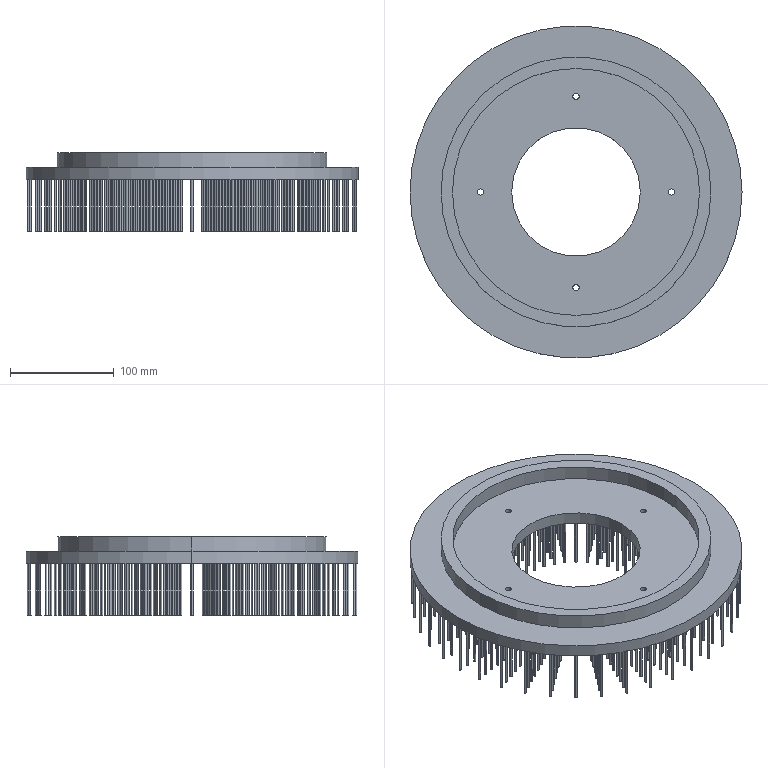Part | NX | features BREP 1 | 1 solid | 1220 faces | box 320 x 320 x 76 mm | volume 1002124 mm3 | cylinder 816 | plane 404 | commonest cylinder face diameters 2 x800 6 x8 124 x2 238 x2 260 x2 320 x2